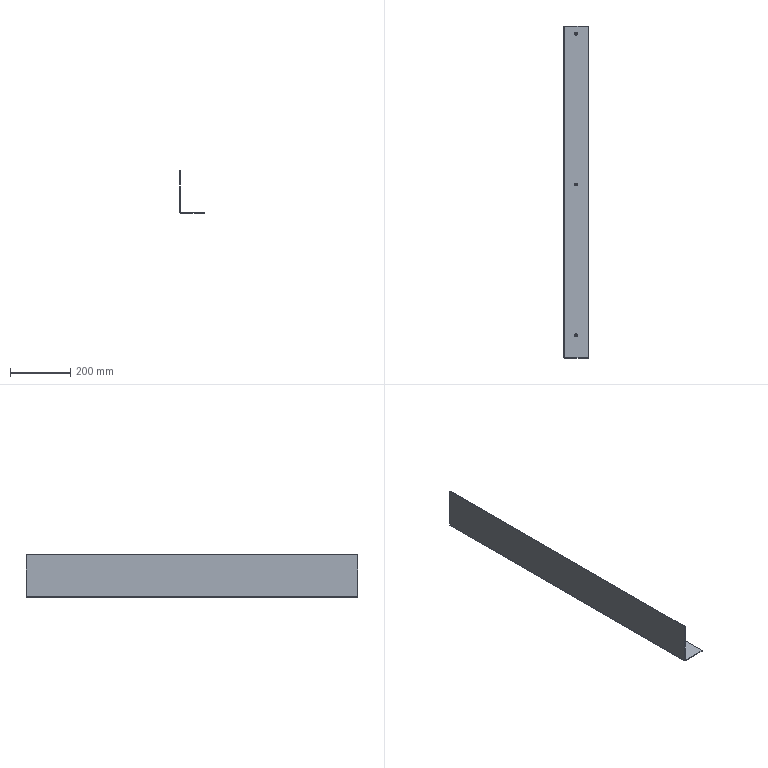Part | STEP file | PN_0006 Partition plate | 1 solid | 16 faces | box 82 x 1100 x 140 mm | volume 481847 mm3 | plane 8 | cone 6 | cylinder 2 | commonest cylinder face diameters 2 x1 6 x1
STEP:
#1=CARTESIAN_POINT('',(0.,0.,0.));
#2=DIRECTION('',(0.,0.,1.));
#3=DIRECTION('',(1.,0.,0.));
#4=AXIS2_PLACEMENT_3D('',#1,#2,#3);
#5=CARTESIAN_POINT('',(43.7,525.,0.));
#6=VERTEX_POINT('',#5);
#7=CARTESIAN_POINT('',(45.7,525.,2.));
#8=VERTEX_POINT('',#7);
#9=CARTESIAN_POINT('',(45.7,525.,2.));
#10=DIRECTION('',(0.7071,0.,0.7071));
#11=VECTOR('',#10,1.);
#12=LINE('',#9,#11);
#13=CARTESIAN_POINT('',(41.,525.,2.));
#14=DIRECTION('',(0.,0.,1.));
#15=DIRECTION('',(1.,0.,0.));
#16=AXIS2_PLACEMENT_3D('',#13,#14,#15);
#17=CONICAL_SURFACE('',#16,4.7,0.7854);
#18=CARTESIAN_POINT('',(6.283,0.));
#19=DIRECTION('',(0.,1.));
#20=VECTOR('',#19,1.);
#21=LINE('',#18,#20);
#22=(GEOMETRIC_REPRESENTATION_CONTEXT(2)PARAMETRIC_REPRESENTATION_CONTEXT()REPRESENTATION_CONTEXT('',''));
#23=DEFINITIONAL_REPRESENTATION('',(#21),#22);
#24=PCURVE('',#17,#23);
#25=CARTESIAN_POINT('',(41.,525.,2.));
#26=DIRECTION('',(0.,0.,1.));
#27=DIRECTION('',(1.,0.,0.));
#28=AXIS2_PLACEMENT_3D('',#25,#26,#27);
#29=CONICAL_SURFACE('',#28,4.7,0.7854);
#30=CARTESIAN_POINT('',(0.,0.));
#31=DIRECTION('',(0.,1.));
#32=VECTOR('',#31,1.);
#33=LINE('',#30,#32);
#34=(GEOMETRIC_REPRESENTATION_CONTEXT(2)PARAMETRIC_REPRESENTATION_CONTEXT()REPRESENTATION_CONTEXT('',''));
#35=DEFINITIONAL_REPRESENTATION('',(#33),#34);
#36=PCURVE('',#29,#35);
#37=SURFACE_CURVE('',#12,(#24,#36),.PCURVE_S1.);
#38=EDGE_CURVE('',#6,#8,#37,.T.);
#39=ORIENTED_EDGE('',*,*,#38,.T.);
#40=CARTESIAN_POINT('',(36.3,525.,2.));
#41=VERTEX_POINT('',#40);
#42=CARTESIAN_POINT('',(41.,525.,2.));
#43=DIRECTION('',(0.,0.,1.));
#44=DIRECTION('',(1.,0.,0.));
#45=AXIS2_PLACEMENT_3D('',#42,#43,#44);
#46=CIRCLE('',#45,4.7);
#47=CARTESIAN_POINT('',(0.,0.));
#48=DIRECTION('',(1.,0.));
#49=VECTOR('',#48,1.);
#50=LINE('',#47,#49);
#51=(GEOMETRIC_REPRESENTATION_CONTEXT(2)PARAMETRIC_REPRESENTATION_CONTEXT()REPRESENTATION_CONTEXT('',''));
#52=DEFINITIONAL_REPRESENTATION('',(#50),#51);
#53=PCURVE('',#17,#52);
#54=CARTESIAN_POINT('',(82.,550.,2.));
#55=DIRECTION('',(0.,0.,-1.));
#56=DIRECTION('',(-1.,0.,0.));
#57=AXIS2_PLACEMENT_3D('',#54,#55,#56);
#58=PLANE('',#57);
#59=CARTESIAN_POINT('',(36.3,-25.));
#60=CARTESIAN_POINT('',(36.3,-16.859));
#61=CARTESIAN_POINT('',(43.35,-20.93));
#62=CARTESIAN_POINT('',(50.4,-25.));
#63=CARTESIAN_POINT('',(43.35,-29.07));
#64=CARTESIAN_POINT('',(36.3,-33.141));
#65=CARTESIAN_POINT('',(36.3,-25.));
#66=(BOUNDED_CURVE()B_SPLINE_CURVE(2,(#59,#60,#61,#62,#63,#64,#65),.UNSPECIFIED.,.T.,.F.)B_SPLINE_CURVE_WITH_KNOTS((1,2,2,2,2,1),(-2.094,0.,2.094,4.189,6.283,8.378),.UNSPECIFIED.)CURVE()GEOMETRIC_REPRESENTATION_ITEM()RATIONAL_B_SPLINE_CURVE((1.,0.5,1.,0.5,1.,0.5,1.))REPRESENTATION_ITEM(''));
#67=(GEOMETRIC_REPRESENTATION_CONTEXT(2)PARAMETRIC_REPRESENTATION_CONTEXT()REPRESENTATION_CONTEXT('',''));
#68=DEFINITIONAL_REPRESENTATION('',(#66),#67);
#69=PCURVE('',#58,#68);
#70=SURFACE_CURVE('',#46,(#53,#69),.PCURVE_S1.);
#71=EDGE_CURVE('',#41,#8,#70,.T.);
#72=ORIENTED_EDGE('',*,*,#71,.F.);
#73=CARTESIAN_POINT('',(38.3,525.,0.));
#74=VERTEX_POINT('',#73);
#75=CARTESIAN_POINT('',(36.3,525.,2.));
#76=DIRECTION('',(-0.7071,0.,0.7071));
#77=VECTOR('',#76,1.);
#78=LINE('',#75,#77);
#79=CARTESIAN_POINT('',(3.142,0.));
#80=DIRECTION('',(0.,1.));
#81=VECTOR('',#80,1.);
#82=LINE('',#79,#81);
#83=(GEOMETRIC_REPRESENTATION_CONTEXT(2)PARAMETRIC_REPRESENTATION_CONTEXT()REPRESENTATION_CONTEXT('',''));
#84=DEFINITIONAL_REPRESENTATION('',(#82),#83);
#85=PCURVE('',#17,#84);
#86=CARTESIAN_POINT('',(3.142,0.));
#87=DIRECTION('',(0.,1.));
#88=VECTOR('',#87,1.);
#89=LINE('',#86,#88);
#90=(GEOMETRIC_REPRESENTATION_CONTEXT(2)PARAMETRIC_REPRESENTATION_CONTEXT()REPRESENTATION_CONTEXT('',''));
#91=DEFINITIONAL_REPRESENTATION('',(#89),#90);
#92=PCURVE('',#29,#91);
#93=SURFACE_CURVE('',#78,(#85,#92),.PCURVE_S1.);
#94=EDGE_CURVE('',#74,#41,#93,.T.);
#95=ORIENTED_EDGE('',*,*,#94,.F.);
#96=CARTESIAN_POINT('',(41.,525.,0.));
#97=DIRECTION('',(0.,0.,1.));
#98=DIRECTION('',(1.,0.,0.));
#99=AXIS2_PLACEMENT_3D('',#96,#97,#98);
#100=CIRCLE('',#99,2.7);
#101=CARTESIAN_POINT('',(0.,-2.));
#102=DIRECTION('',(1.,0.));
#103=VECTOR('',#102,1.);
#104=LINE('',#101,#103);
#105=(GEOMETRIC_REPRESENTATION_CONTEXT(2)PARAMETRIC_REPRESENTATION_CONTEXT()REPRESENTATION_CONTEXT('',''));
#106=DEFINITIONAL_REPRESENTATION('',(#104),#105);
#107=PCURVE('',#17,#106);
#108=CARTESIAN_POINT('',(3.,550.,0.));
#109=DIRECTION('',(0.,0.,1.));
#110=DIRECTION('',(1.,0.,0.));
#111=AXIS2_PLACEMENT_3D('',#108,#109,#110);
#112=PLANE('',#111);
#113=CARTESIAN_POINT('',(38.,-25.));
#114=DIRECTION('',(1.,0.));
#115=AXIS2_PLACEMENT_2D('',#113,#114);
#116=CIRCLE('',#115,2.7);
#117=(GEOMETRIC_REPRESENTATION_CONTEXT(2)PARAMETRIC_REPRESENTATION_CONTEXT()REPRESENTATION_CONTEXT('',''));
#118=DEFINITIONAL_REPRESENTATION('',(#116),#117);
#119=PCURVE('',#112,#118);
#120=SURFACE_CURVE('',#100,(#107,#119),.PCURVE_S1.);
#121=EDGE_CURVE('',#74,#6,#120,.T.);
#122=ORIENTED_EDGE('',*,*,#121,.T.);
#123=EDGE_LOOP('',(#39,#72,#95,#122));
#124=FACE_BOUND('',#123,.F.);
#125=ADVANCED_FACE('',(#124),#17,.F.);
#126=CARTESIAN_POINT('',(43.7,25.,0.));
#127=VERTEX_POINT('',#126);
#128=CARTESIAN_POINT('',(45.7,25.,2.));
#129=VERTEX_POINT('',#128);
#130=CARTESIAN_POINT('',(45.7,25.,2.));
#131=DIRECTION('',(0.7071,0.,0.7071));
#132=VECTOR('',#131,1.);
#133=LINE('',#130,#132);
#134=CARTESIAN_POINT('',(41.,25.,2.));
#135=DIRECTION('',(0.,0.,1.));
#136=DIRECTION('',(1.,0.,0.));
#137=AXIS2_PLACEMENT_3D('',#134,#135,#136);
#138=CONICAL_SURFACE('',#137,4.7,0.7854);
#139=CARTESIAN_POINT('',(6.283,0.));
#140=DIRECTION('',(0.,1.));
#141=VECTOR('',#140,1.);
#142=LINE('',#139,#141);
#143=(GEOMETRIC_REPRESENTATION_CONTEXT(2)PARAMETRIC_REPRESENTATION_CONTEXT()REPRESENTATION_CONTEXT('',''));
#144=DEFINITIONAL_REPRESENTATION('',(#142),#143);
#145=PCURVE('',#138,#144);
#146=CARTESIAN_POINT('',(41.,25.,2.));
#147=DIRECTION('',(0.,0.,1.));
#148=DIRECTION('',(1.,0.,0.));
#149=AXIS2_PLACEMENT_3D('',#146,#147,#148);
#150=CONICAL_SURFACE('',#149,4.7,0.7854);
#151=CARTESIAN_POINT('',(0.,0.));
#152=DIRECTION('',(0.,1.));
#153=VECTOR('',#152,1.);
#154=LINE('',#151,#153);
#155=(GEOMETRIC_REPRESENTATION_CONTEXT(2)PARAMETRIC_REPRESENTATION_CONTEXT()REPRESENTATION_CONTEXT('',''));
#156=DEFINITIONAL_REPRESENTATION('',(#154),#155);
#157=PCURVE('',#150,#156);
#158=SURFACE_CURVE('',#133,(#145,#157),.PCURVE_S1.);
#159=EDGE_CURVE('',#127,#129,#158,.T.);
#160=ORIENTED_EDGE('',*,*,#159,.T.);
#161=CARTESIAN_POINT('',(36.3,25.,2.));
#162=VERTEX_POINT('',#161);
#163=CARTESIAN_POINT('',(41.,25.,2.));
#164=DIRECTION('',(0.,0.,1.));
#165=DIRECTION('',(1.,0.,0.));
#166=AXIS2_PLACEMENT_3D('',#163,#164,#165);
#167=CIRCLE('',#166,4.7);
#168=CARTESIAN_POINT('',(0.,0.));
#169=DIRECTION('',(1.,0.));
#170=VECTOR('',#169,1.);
#171=LINE('',#168,#170);
#172=(GEOMETRIC_REPRESENTATION_CONTEXT(2)PARAMETRIC_REPRESENTATION_CONTEXT()REPRESENTATION_CONTEXT('',''));
#173=DEFINITIONAL_REPRESENTATION('',(#171),#172);
#174=PCURVE('',#138,#173);
#175=CARTESIAN_POINT('',(36.3,-525.));
#176=CARTESIAN_POINT('',(36.3,-516.859));
#177=CARTESIAN_POINT('',(43.35,-520.93));
#178=CARTESIAN_POINT('',(50.4,-525.));
#179=CARTESIAN_POINT('',(43.35,-529.07));
#180=CARTESIAN_POINT('',(36.3,-533.141));
#181=CARTESIAN_POINT('',(36.3,-525.));
#182=(BOUNDED_CURVE()B_SPLINE_CURVE(2,(#175,#176,#177,#178,#179,#180,#181),.UNSPECIFIED.,.T.,.F.)B_SPLINE_CURVE_WITH_KNOTS((1,2,2,2,2,1),(-2.094,0.,2.094,4.189,6.283,8.378),.UNSPECIFIED.)CURVE()GEOMETRIC_REPRESENTATION_ITEM()RATIONAL_B_SPLINE_CURVE((1.,0.5,1.,0.5,1.,0.5,1.))REPRESENTATION_ITEM(''));
#183=(GEOMETRIC_REPRESENTATION_CONTEXT(2)PARAMETRIC_REPRESENTATION_CONTEXT()REPRESENTATION_CONTEXT('',''));
#184=DEFINITIONAL_REPRESENTATION('',(#182),#183);
#185=PCURVE('',#58,#184);
#186=SURFACE_CURVE('',#167,(#174,#185),.PCURVE_S1.);
#187=EDGE_CURVE('',#162,#129,#186,.T.);
#188=ORIENTED_EDGE('',*,*,#187,.F.);
#189=CARTESIAN_POINT('',(38.3,25.,0.));
#190=VERTEX_POINT('',#189);
#191=CARTESIAN_POINT('',(36.3,25.,2.));
#192=DIRECTION('',(-0.7071,0.,0.7071));
#193=VECTOR('',#192,1.);
#194=LINE('',#191,#193);
#195=CARTESIAN_POINT('',(3.142,0.));
#196=DIRECTION('',(0.,1.));
#197=VECTOR('',#196,1.);
#198=LINE('',#195,#197);
#199=(GEOMETRIC_REPRESENTATION_CONTEXT(2)PARAMETRIC_REPRESENTATION_CONTEXT()REPRESENTATION_CONTEXT('',''));
#200=DEFINITIONAL_REPRESENTATION('',(#198),#199);
#201=PCURVE('',#138,#200);
#202=CARTESIAN_POINT('',(3.142,0.));
#203=DIRECTION('',(0.,1.));
#204=VECTOR('',#203,1.);
#205=LINE('',#202,#204);
#206=(GEOMETRIC_REPRESENTATION_CONTEXT(2)PARAMETRIC_REPRESENTATION_CONTEXT()REPRESENTATION_CONTEXT('',''));
#207=DEFINITIONAL_REPRESENTATION('',(#205),#206);
#208=PCURVE('',#150,#207);
#209=SURFACE_CURVE('',#194,(#201,#208),.PCURVE_S1.);
#210=EDGE_CURVE('',#190,#162,#209,.T.);
#211=ORIENTED_EDGE('',*,*,#210,.F.);
#212=CARTESIAN_POINT('',(41.,25.,0.));
#213=DIRECTION('',(0.,0.,1.));
#214=DIRECTION('',(1.,0.,0.));
#215=AXIS2_PLACEMENT_3D('',#212,#213,#214);
#216=CIRCLE('',#215,2.7);
#217=CARTESIAN_POINT('',(0.,-2.));
#218=DIRECTION('',(1.,0.));
#219=VECTOR('',#218,1.);
#220=LINE('',#217,#219);
#221=(GEOMETRIC_REPRESENTATION_CONTEXT(2)PARAMETRIC_REPRESENTATION_CONTEXT()REPRESENTATION_CONTEXT('',''));
#222=DEFINITIONAL_REPRESENTATION('',(#220),#221);
#223=PCURVE('',#138,#222);
#224=CARTESIAN_POINT('',(38.,-525.));
#225=DIRECTION('',(1.,0.));
#226=AXIS2_PLACEMENT_2D('',#224,#225);
#227=CIRCLE('',#226,2.7);
#228=(GEOMETRIC_REPRESENTATION_CONTEXT(2)PARAMETRIC_REPRESENTATION_CONTEXT()REPRESENTATION_CONTEXT('',''));
#229=DEFINITIONAL_REPRESENTATION('',(#227),#228);
#230=PCURVE('',#112,#229);
#231=SURFACE_CURVE('',#216,(#223,#230),.PCURVE_S1.);
#232=EDGE_CURVE('',#190,#127,#231,.T.);
#233=ORIENTED_EDGE('',*,*,#232,.T.);
#234=EDGE_LOOP('',(#160,#188,#211,#233));
#235=FACE_BOUND('',#234,.F.);
#236=ADVANCED_FACE('',(#235),#138,.F.);
#237=CARTESIAN_POINT('',(43.7,-475.,0.));
#238=VERTEX_POINT('',#237);
#239=CARTESIAN_POINT('',(45.7,-475.,2.));
#240=VERTEX_POINT('',#239);
#241=CARTESIAN_POINT('',(45.7,-475.,2.));
#242=DIRECTION('',(0.7071,0.,0.7071));
#243=VECTOR('',#242,1.);
#244=LINE('',#241,#243);
#245=CARTESIAN_POINT('',(41.,-475.,2.));
#246=DIRECTION('',(0.,0.,1.));
#247=DIRECTION('',(1.,0.,0.));
#248=AXIS2_PLACEMENT_3D('',#245,#246,#247);
#249=CONICAL_SURFACE('',#248,4.7,0.7854);
#250=CARTESIAN_POINT('',(6.283,0.));
#251=DIRECTION('',(0.,1.));
#252=VECTOR('',#251,1.);
#253=LINE('',#250,#252);
#254=(GEOMETRIC_REPRESENTATION_CONTEXT(2)PARAMETRIC_REPRESENTATION_CONTEXT()REPRESENTATION_CONTEXT('',''));
#255=DEFINITIONAL_REPRESENTATION('',(#253),#254);
#256=PCURVE('',#249,#255);
#257=CARTESIAN_POINT('',(41.,-475.,2.));
#258=DIRECTION('',(0.,0.,1.));
#259=DIRECTION('',(1.,0.,0.));
#260=AXIS2_PLACEMENT_3D('',#257,#258,#259);
#261=CONICAL_SURFACE('',#260,4.7,0.7854);
#262=CARTESIAN_POINT('',(0.,0.));
#263=DIRECTION('',(0.,1.));
#264=VECTOR('',#263,1.);
#265=LINE('',#262,#264);
#266=(GEOMETRIC_REPRESENTATION_CONTEXT(2)PARAMETRIC_REPRESENTATION_CONTEXT()REPRESENTATION_CONTEXT('',''));
#267=DEFINITIONAL_REPRESENTATION('',(#265),#266);
#268=PCURVE('',#261,#267);
#269=SURFACE_CURVE('',#244,(#256,#268),.PCURVE_S1.);
#270=EDGE_CURVE('',#238,#240,#269,.T.);
#271=ORIENTED_EDGE('',*,*,#270,.T.);
#272=CARTESIAN_POINT('',(36.3,-475.,2.));
#273=VERTEX_POINT('',#272);
#274=CARTESIAN_POINT('',(41.,-475.,2.));
#275=DIRECTION('',(0.,0.,1.));
#276=DIRECTION('',(1.,0.,0.));
#277=AXIS2_PLACEMENT_3D('',#274,#275,#276);
#278=CIRCLE('',#277,4.7);
#279=CARTESIAN_POINT('',(0.,0.));
#280=DIRECTION('',(1.,0.));
#281=VECTOR('',#280,1.);
#282=LINE('',#279,#281);
#283=(GEOMETRIC_REPRESENTATION_CONTEXT(2)PARAMETRIC_REPRESENTATION_CONTEXT()REPRESENTATION_CONTEXT('',''));
#284=DEFINITIONAL_REPRESENTATION('',(#282),#283);
#285=PCURVE('',#249,#284);
#286=CARTESIAN_POINT('',(36.3,-1025.));
#287=CARTESIAN_POINT('',(36.3,-1016.859));
#288=CARTESIAN_POINT('',(43.35,-1020.93));
#289=CARTESIAN_POINT('',(50.4,-1025.));
#290=CARTESIAN_POINT('',(43.35,-1029.07));
#291=CARTESIAN_POINT('',(36.3,-1033.141));
#292=CARTESIAN_POINT('',(36.3,-1025.));
#293=(BOUNDED_CURVE()B_SPLINE_CURVE(2,(#286,#287,#288,#289,#290,#291,#292),.UNSPECIFIED.,.T.,.F.)B_SPLINE_CURVE_WITH_KNOTS((1,2,2,2,2,1),(-2.094,0.,2.094,4.189,6.283,8.378),.UNSPECIFIED.)CURVE()GEOMETRIC_REPRESENTATION_ITEM()RATIONAL_B_SPLINE_CURVE((1.,0.5,1.,0.5,1.,0.5,1.))REPRESENTATION_ITEM(''));
#294=(GEOMETRIC_REPRESENTATION_CONTEXT(2)PARAMETRIC_REPRESENTATION_CONTEXT()REPRESENTATION_CONTEXT('',''));
#295=DEFINITIONAL_REPRESENTATION('',(#293),#294);
#296=PCURVE('',#58,#295);
#297=SURFACE_CURVE('',#278,(#285,#296),.PCURVE_S1.);
#298=EDGE_CURVE('',#273,#240,#297,.T.);
#299=ORIENTED_EDGE('',*,*,#298,.F.);
#300=CARTESIAN_POINT('',(38.3,-475.,0.));
#301=VERTEX_POINT('',#300);
#302=CARTESIAN_POINT('',(36.3,-475.,2.));
#303=DIRECTION('',(-0.7071,0.,0.7071));
#304=VECTOR('',#303,1.);
#305=LINE('',#302,#304);
#306=CARTESIAN_POINT('',(3.142,0.));
#307=DIRECTION('',(0.,1.));
#308=VECTOR('',#307,1.);
#309=LINE('',#306,#308);
#310=(GEOMETRIC_REPRESENTATION_CONTEXT(2)PARAMETRIC_REPRESENTATION_CONTEXT()REPRESENTATION_CONTEXT('',''));
#311=DEFINITIONAL_REPRESENTATION('',(#309),#310);
#312=PCURVE('',#249,#311);
#313=CARTESIAN_POINT('',(3.142,0.));
#314=DIRECTION('',(0.,1.));
#315=VECTOR('',#314,1.);
#316=LINE('',#313,#315);
#317=(GEOMETRIC_REPRESENTATION_CONTEXT(2)PARAMETRIC_REPRESENTATION_CONTEXT()REPRESENTATION_CONTEXT('',''));
#318=DEFINITIONAL_REPRESENTATION('',(#316),#317);
#319=PCURVE('',#261,#318);
#320=SURFACE_CURVE('',#305,(#312,#319),.PCURVE_S1.);
#321=EDGE_CURVE('',#301,#273,#320,.T.);
#322=ORIENTED_EDGE('',*,*,#321,.F.);
#323=CARTESIAN_POINT('',(41.,-475.,0.));
#324=DIRECTION('',(0.,0.,1.));
#325=DIRECTION('',(1.,0.,0.));
#326=AXIS2_PLACEMENT_3D('',#323,#324,#325);
#327=CIRCLE('',#326,2.7);
#328=CARTESIAN_POINT('',(0.,-2.));
#329=DIRECTION('',(1.,0.));
#330=VECTOR('',#329,1.);
#331=LINE('',#328,#330);
#332=(GEOMETRIC_REPRESENTATION_CONTEXT(2)PARAMETRIC_REPRESENTATION_CONTEXT()REPRESENTATION_CONTEXT('',''));
#333=DEFINITIONAL_REPRESENTATION('',(#331),#332);
#334=PCURVE('',#249,#333);
#335=CARTESIAN_POINT('',(38.,-1025.));
#336=DIRECTION('',(1.,0.));
#337=AXIS2_PLACEMENT_2D('',#335,#336);
#338=CIRCLE('',#337,2.7);
#339=(GEOMETRIC_REPRESENTATION_CONTEXT(2)PARAMETRIC_REPRESENTATION_CONTEXT()REPRESENTATION_CONTEXT('',''));
#340=DEFINITIONAL_REPRESENTATION('',(#338),#339);
#341=PCURVE('',#112,#340);
#342=SURFACE_CURVE('',#327,(#334,#341),.PCURVE_S1.);
#343=EDGE_CURVE('',#301,#238,#342,.T.);
#344=ORIENTED_EDGE('',*,*,#343,.T.);
#345=EDGE_LOOP('',(#271,#299,#322,#344));
#346=FACE_BOUND('',#345,.F.);
#347=ADVANCED_FACE('',(#346),#249,.F.);
#348=CARTESIAN_POINT('',(41.,525.,0.));
#349=DIRECTION('',(0.,0.,1.));
#350=DIRECTION('',(1.,0.,0.));
#351=AXIS2_PLACEMENT_3D('',#348,#349,#350);
#352=CIRCLE('',#351,2.7);
#353=CARTESIAN_POINT('',(38.,-25.));
#354=DIRECTION('',(1.,0.));
#355=AXIS2_PLACEMENT_2D('',#353,#354);
#356=CIRCLE('',#355,2.7);
#357=(GEOMETRIC_REPRESENTATION_CONTEXT(2)PARAMETRIC_REPRESENTATION_CONTEXT()REPRESENTATION_CONTEXT('',''));
#358=DEFINITIONAL_REPRESENTATION('',(#356),#357);
#359=PCURVE('',#112,#358);
#360=CARTESIAN_POINT('',(0.,-2.));
#361=DIRECTION('',(1.,0.));
#362=VECTOR('',#361,1.);
#363=LINE('',#360,#362);
#364=(GEOMETRIC_REPRESENTATION_CONTEXT(2)PARAMETRIC_REPRESENTATION_CONTEXT()REPRESENTATION_CONTEXT('',''));
#365=DEFINITIONAL_REPRESENTATION('',(#363),#364);
#366=PCURVE('',#29,#365);
#367=SURFACE_CURVE('',#352,(#359,#366),.PCURVE_S1.);
#368=EDGE_CURVE('',#6,#74,#367,.T.);
#369=ORIENTED_EDGE('',*,*,#368,.T.);
#370=ORIENTED_EDGE('',*,*,#121,.T.);
#371=EDGE_LOOP('',(#369,#370));
#372=FACE_BOUND('',#371,.T.);
#373=CARTESIAN_POINT('',(41.,25.,0.));
#374=DIRECTION('',(0.,0.,1.));
#375=DIRECTION('',(1.,0.,0.));
#376=AXIS2_PLACEMENT_3D('',#373,#374,#375);
#377=CIRCLE('',#376,2.7);
#378=CARTESIAN_POINT('',(38.,-525.));
#379=DIRECTION('',(1.,0.));
#380=AXIS2_PLACEMENT_2D('',#378,#379);
#381=CIRCLE('',#380,2.7);
#382=(GEOMETRIC_REPRESENTATION_CONTEXT(2)PARAMETRIC_REPRESENTATION_CONTEXT()REPRESENTATION_CONTEXT('',''));
#383=DEFINITIONAL_REPRESENTATION('',(#381),#382);
#384=PCURVE('',#112,#383);
#385=CARTESIAN_POINT('',(0.,-2.));
#386=DIRECTION('',(1.,0.));
#387=VECTOR('',#386,1.);
#388=LINE('',#385,#387);
#389=(GEOMETRIC_REPRESENTATION_CONTEXT(2)PARAMETRIC_REPRESENTATION_CONTEXT()REPRESENTATION_CONTEXT('',''));
#390=DEFINITIONAL_REPRESENTATION('',(#388),#389);
#391=PCURVE('',#150,#390);
#392=SURFACE_CURVE('',#377,(#384,#391),.PCURVE_S1.);
#393=EDGE_CURVE('',#127,#190,#392,.T.);
#394=ORIENTED_EDGE('',*,*,#393,.T.);
#395=ORIENTED_EDGE('',*,*,#232,.T.);
#396=EDGE_LOOP('',(#394,#395));
#397=FACE_BOUND('',#396,.T.);
#398=CARTESIAN_POINT('',(41.,-475.,0.));
#399=DIRECTION('',(0.,0.,1.));
#400=DIRECTION('',(1.,0.,0.));
#401=AXIS2_PLACEMENT_3D('',#398,#399,#400);
#402=CIRCLE('',#401,2.7);
#403=CARTESIAN_POINT('',(38.,-1025.));
#404=DIRECTION('',(1.,0.));
#405=AXIS2_PLACEMENT_2D('',#403,#404);
#406=CIRCLE('',#405,2.7);
#407=(GEOMETRIC_REPRESENTATION_CONTEXT(2)PARAMETRIC_REPRESENTATION_CONTEXT()REPRESENTATION_CONTEXT('',''));
#408=DEFINITIONAL_REPRESENTATION('',(#406),#407);
#409=PCURVE('',#112,#408);
#410=CARTESIAN_POINT('',(0.,-2.));
#411=DIRECTION('',(1.,0.));
#412=VECTOR('',#411,1.);
#413=LINE('',#410,#412);
#414=(GEOMETRIC_REPRESENTATION_CONTEXT(2)PARAMETRIC_REPRESENTATION_CONTEXT()REPRESENTATION_CONTEXT('',''));
#415=DEFINITIONAL_REPRESENTATION('',(#413),#414);
#416=PCURVE('',#261,#415);
#417=SURFACE_CURVE('',#402,(#409,#416),.PCURVE_S1.);
#418=EDGE_CURVE('',#238,#301,#417,.T.);
#419=ORIENTED_EDGE('',*,*,#418,.T.);
#420=ORIENTED_EDGE('',*,*,#343,.T.);
#421=EDGE_LOOP('',(#419,#420));
#422=FACE_BOUND('',#421,.T.);
#423=CARTESIAN_POINT('',(82.,-550.,0.));
#424=VERTEX_POINT('',#423);
#425=CARTESIAN_POINT('',(3.,-550.,0.));
#426=VERTEX_POINT('',#425);
#427=CARTESIAN_POINT('',(3.,-550.,0.));
#428=DIRECTION('',(-1.,0.,0.));
#429=VECTOR('',#428,1.);
#430=LINE('',#427,#429);
#431=CARTESIAN_POINT('',(0.,-1100.));
#432=DIRECTION('',(-1.,0.));
#433=VECTOR('',#432,1.);
#434=LINE('',#431,#433);
#435=(GEOMETRIC_REPRESENTATION_CONTEXT(2)PARAMETRIC_REPRESENTATION_CONTEXT()REPRESENTATION_CONTEXT('',''));
#436=DEFINITIONAL_REPRESENTATION('',(#434),#435);
#437=PCURVE('',#112,#436);
#438=CARTESIAN_POINT('',(3.,-550.,3.));
#439=DIRECTION('',(0.,-1.,0.));
#440=DIRECTION('',(0.,0.,-1.));
#441=AXIS2_PLACEMENT_3D('',#438,#439,#440);
#442=PLANE('',#441);
#443=CARTESIAN_POINT('',(3.,0.));
#444=DIRECTION('',(0.,-1.));
#445=VECTOR('',#444,1.);
#446=LINE('',#443,#445);
#447=(GEOMETRIC_REPRESENTATION_CONTEXT(2)PARAMETRIC_REPRESENTATION_CONTEXT()REPRESENTATION_CONTEXT('',''));
#448=DEFINITIONAL_REPRESENTATION('',(#446),#447);
#449=PCURVE('',#442,#448);
#450=SURFACE_CURVE('',#430,(#437,#449),.PCURVE_S1.);
#451=EDGE_CURVE('',#424,#426,#450,.T.);
#452=ORIENTED_EDGE('',*,*,#451,.T.);
#453=CARTESIAN_POINT('',(3.,550.,0.));
#454=VERTEX_POINT('',#453);
#455=CARTESIAN_POINT('',(3.,550.,0.));
#456=DIRECTION('',(0.,-1.,0.));
#457=VECTOR('',#456,1.);
#458=LINE('',#455,#457);
#459=CARTESIAN_POINT('',(0.,0.));
#460=DIRECTION('',(0.,-1.));
#461=VECTOR('',#460,1.);
#462=LINE('',#459,#461);
#463=(GEOMETRIC_REPRESENTATION_CONTEXT(2)PARAMETRIC_REPRESENTATION_CONTEXT()REPRESENTATION_CONTEXT('',''));
#464=DEFINITIONAL_REPRESENTATION('',(#462),#463);
#465=PCURVE('',#112,#464);
#466=CARTESIAN_POINT('',(3.,550.,3.));
#467=DIRECTION('',(0.,-1.,0.));
#468=DIRECTION('',(0.,0.,-1.));
#469=AXIS2_PLACEMENT_3D('',#466,#467,#468);
#470=CYLINDRICAL_SURFACE('',#469,3.);
#471=CARTESIAN_POINT('',(6.283,0.));
#472=DIRECTION('',(0.,1.));
#473=VECTOR('',#472,1.);
#474=LINE('',#471,#473);
#475=(GEOMETRIC_REPRESENTATION_CONTEXT(2)PARAMETRIC_REPRESENTATION_CONTEXT()REPRESENTATION_CONTEXT('',''));
#476=DEFINITIONAL_REPRESENTATION('',(#474),#475);
#477=PCURVE('',#470,#476);
#478=SURFACE_CURVE('',#458,(#465,#477),.PCURVE_S1.);
#479=EDGE_CURVE('',#454,#426,#478,.T.);
#480=ORIENTED_EDGE('',*,*,#479,.F.);
#481=CARTESIAN_POINT('',(82.,550.,0.));
#482=VERTEX_POINT('',#481);
#483=CARTESIAN_POINT('',(3.,550.,0.));
#484=DIRECTION('',(-1.,0.,0.));
#485=VECTOR('',#484,1.);
#486=LINE('',#483,#485);
#487=CARTESIAN_POINT('',(0.,0.));
#488=DIRECTION('',(-1.,0.));
#489=VECTOR('',#488,1.);
#490=LINE('',#487,#489);
#491=(GEOMETRIC_REPRESENTATION_CONTEXT(2)PARAMETRIC_REPRESENTATION_CONTEXT()REPRESENTATION_CONTEXT('',''));
#492=DEFINITIONAL_REPRESENTATION('',(#490),#491);
#493=PCURVE('',#112,#492);
#494=CARTESIAN_POINT('',(3.,550.,3.));
#495=DIRECTION('',(0.,-1.,0.));
#496=DIRECTION('',(0.,0.,-1.));
#497=AXIS2_PLACEMENT_3D('',#494,#495,#496);
#498=PLANE('',#497);
#499=CARTESIAN_POINT('',(3.,0.));
#500=DIRECTION('',(0.,-1.));
#501=VECTOR('',#500,1.);
#502=LINE('',#499,#501);
#503=(GEOMETRIC_REPRESENTATION_CONTEXT(2)PARAMETRIC_REPRESENTATION_CONTEXT()REPRESENTATION_CONTEXT('',''));
#504=DEFINITIONAL_REPRESENTATION('',(#502),#503);
#505=PCURVE('',#498,#504);
#506=SURFACE_CURVE('',#486,(#493,#505),.PCURVE_S1.);
#507=EDGE_CURVE('',#482,#454,#506,.T.);
#508=ORIENTED_EDGE('',*,*,#507,.F.);
#509=CARTESIAN_POINT('',(82.,550.,0.));
#510=DIRECTION('',(0.,-1.,0.));
#511=VECTOR('',#510,1.);
#512=LINE('',#509,#511);
#513=CARTESIAN_POINT('',(79.,0.));
#514=DIRECTION('',(0.,-1.));
#515=VECTOR('',#514,1.);
#516=LINE('',#513,#515);
#517=(GEOMETRIC_REPRESENTATION_CONTEXT(2)PARAMETRIC_REPRESENTATION_CONTEXT()REPRESENTATION_CONTEXT('',''));
#518=DEFINITIONAL_REPRESENTATION('',(#516),#517);
#519=PCURVE('',#112,#518);
#520=CARTESIAN_POINT('',(82.,550.,0.));
#521=DIRECTION('',(-1.,0.,0.));
#522=DIRECTION('',(0.,0.,1.));
#523=AXIS2_PLACEMENT_3D('',#520,#521,#522);
#524=PLANE('',#523);
#525=CARTESIAN_POINT('',(0.,0.));
#526=DIRECTION('',(0.,-1.));
#527=VECTOR('',#526,1.);
#528=LINE('',#525,#527);
#529=(GEOMETRIC_REPRESENTATION_CONTEXT(2)PARAMETRIC_REPRESENTATION_CONTEXT()REPRESENTATION_CONTEXT('',''));
#530=DEFINITIONAL_REPRESENTATION('',(#528),#529);
#531=PCURVE('',#524,#530);
#532=SURFACE_CURVE('',#512,(#519,#531),.PCURVE_S1.);
#533=EDGE_CURVE('',#482,#424,#532,.T.);
#534=ORIENTED_EDGE('',*,*,#533,.T.);
#535=EDGE_LOOP('',(#452,#480,#508,#534));
#536=FACE_BOUND('',#535,.T.);
#537=ADVANCED_FACE('',(#372,#397,#422,#536),#112,.F.);
#538=CARTESIAN_POINT('',(0.,-550.,140.));
#539=VERTEX_POINT('',#538);
#540=CARTESIAN_POINT('',(2.,-550.,140.));
#541=VERTEX_POINT('',#540);
#542=CARTESIAN_POINT('',(2.,-550.,140.));
#543=DIRECTION('',(1.,0.,0.));
#544=VECTOR('',#543,1.);
#545=LINE('',#542,#544);
#546=CARTESIAN_POINT('',(2.,550.,140.));
#547=DIRECTION('',(0.,0.,-1.));
#548=DIRECTION('',(-1.,0.,0.));
#549=AXIS2_PLACEMENT_3D('',#546,#547,#548);
#550=PLANE('',#549);
#551=CARTESIAN_POINT('',(0.,-1100.));
#552=DIRECTION('',(-1.,0.));
#553=VECTOR('',#552,1.);
#554=LINE('',#551,#553);
#555=(GEOMETRIC_REPRESENTATION_CONTEXT(2)PARAMETRIC_REPRESENTATION_CONTEXT()REPRESENTATION_CONTEXT('',''));
#556=DEFINITIONAL_REPRESENTATION('',(#554),#555);
#557=PCURVE('',#550,#556);
#558=CARTESIAN_POINT('',(-137.,-1.));
#559=DIRECTION('',(0.,1.));
#560=VECTOR('',#559,1.);
#561=LINE('',#558,#560);
#562=(GEOMETRIC_REPRESENTATION_CONTEXT(2)PARAMETRIC_REPRESENTATION_CONTEXT()REPRESENTATION_CONTEXT('',''));
#563=DEFINITIONAL_REPRESENTATION('',(#561),#562);
#564=PCURVE('',#442,#563);
#565=SURFACE_CURVE('',#545,(#557,#564),.PCURVE_S1.);
#566=EDGE_CURVE('',#539,#541,#565,.T.);
#567=ORIENTED_EDGE('',*,*,#566,.T.);
#568=CARTESIAN_POINT('',(2.,550.,140.));
#569=VERTEX_POINT('',#568);
#570=CARTESIAN_POINT('',(2.,550.,140.));
#571=DIRECTION('',(0.,-1.,0.));
#572=VECTOR('',#571,1.);
#573=LINE('',#570,#572);
#574=CARTESIAN_POINT('',(0.,0.));
#575=DIRECTION('',(0.,-1.));
#576=VECTOR('',#575,1.);
#577=LINE('',#574,#576);
#578=(GEOMETRIC_REPRESENTATION_CONTEXT(2)PARAMETRIC_REPRESENTATION_CONTEXT()REPRESENTATION_CONTEXT('',''));
#579=DEFINITIONAL_REPRESENTATION('',(#577),#578);
#580=PCURVE('',#550,#579);
#581=CARTESIAN_POINT('',(2.,550.,3.));
#582=DIRECTION('',(-1.,0.,0.));
#583=DIRECTION('',(0.,0.,1.));
#584=AXIS2_PLACEMENT_3D('',#581,#582,#583);
#585=PLANE('',#584);
#586=CARTESIAN_POINT('',(137.,0.));
#587=DIRECTION('',(0.,-1.));
#588=VECTOR('',#587,1.);
#589=LINE('',#586,#588);
#590=(GEOMETRIC_REPRESENTATION_CONTEXT(2)PARAMETRIC_REPRESENTATION_CONTEXT()REPRESENTATION_CONTEXT('',''));
#591=DEFINITIONAL_REPRESENTATION('',(#589),#590);
#592=PCURVE('',#585,#591);
#593=SURFACE_CURVE('',#573,(#580,#592),.PCURVE_S1.);
#594=EDGE_CURVE('',#569,#541,#593,.T.);
#595=ORIENTED_EDGE('',*,*,#594,.F.);
#596=CARTESIAN_POINT('',(0.,550.,140.));
#597=VERTEX_POINT('',#596);
#598=CARTESIAN_POINT('',(2.,550.,140.));
#599=DIRECTION('',(1.,0.,0.));
#600=VECTOR('',#599,1.);
#601=LINE('',#598,#600);
#602=CARTESIAN_POINT('',(0.,0.));
#603=DIRECTION('',(-1.,0.));
#604=VECTOR('',#603,1.);
#605=LINE('',#602,#604);
#606=(GEOMETRIC_REPRESENTATION_CONTEXT(2)PARAMETRIC_REPRESENTATION_CONTEXT()REPRESENTATION_CONTEXT('',''));
#607=DEFINITIONAL_REPRESENTATION('',(#605),#606);
#608=PCURVE('',#550,#607);
#609=CARTESIAN_POINT('',(-137.,-1.));
#610=DIRECTION('',(0.,1.));
#611=VECTOR('',#610,1.);
#612=LINE('',#609,#611);
#613=(GEOMETRIC_REPRESENTATION_CONTEXT(2)PARAMETRIC_REPRESENTATION_CONTEXT()REPRESENTATION_CONTEXT('',''));
#614=DEFINITIONAL_REPRESENTATION('',(#612),#613);
#615=PCURVE('',#498,#614);
#616=SURFACE_CURVE('',#601,(#608,#615),.PCURVE_S1.);
#617=EDGE_CURVE('',#597,#569,#616,.T.);
#618=ORIENTED_EDGE('',*,*,#617,.F.);
#619=CARTESIAN_POINT('',(0.,550.,140.));
#620=DIRECTION('',(0.,-1.,0.));
#621=VECTOR('',#620,1.);
#622=LINE('',#619,#621);
#623=CARTESIAN_POINT('',(2.,0.));
#624=DIRECTION('',(0.,-1.));
#625=VECTOR('',#624,1.);
#626=LINE('',#623,#625);
#627=(GEOMETRIC_REPRESENTATION_CONTEXT(2)PARAMETRIC_REPRESENTATION_CONTEXT()REPRESENTATION_CONTEXT('',''));
#628=DEFINITIONAL_REPRESENTATION('',(#626),#627);
#629=PCURVE('',#550,#628);
#630=CARTESIAN_POINT('',(0.,550.,140.));
#631=DIRECTION('',(1.,0.,0.));
#632=DIRECTION('',(0.,0.,-1.));
#633=AXIS2_PLACEMENT_3D('',#630,#631,#632);
#634=PLANE('',#633);
#635=CARTESIAN_POINT('',(0.,0.));
#636=DIRECTION('',(0.,-1.));
#637=VECTOR('',#636,1.);
#638=LINE('',#635,#637);
#639=(GEOMETRIC_REPRESENTATION_CONTEXT(2)PARAMETRIC_REPRESENTATION_CONTEXT()REPRESENTATION_CONTEXT('',''));
#640=DEFINITIONAL_REPRESENTATION('',(#638),#639);
#641=PCURVE('',#634,#640);
#642=SURFACE_CURVE('',#622,(#629,#641),.PCURVE_S1.);
#643=EDGE_CURVE('',#597,#539,#642,.T.);
#644=ORIENTED_EDGE('',*,*,#643,.T.);
#645=EDGE_LOOP('',(#567,#595,#618,#644));
#646=FACE_BOUND('',#645,.T.);
#647=ADVANCED_FACE('',(#646),#550,.F.);
#648=CARTESIAN_POINT('',(2.,-550.,3.));
#649=VERTEX_POINT('',#648);
#650=CARTESIAN_POINT('',(2.,-550.,3.));
#651=DIRECTION('',(0.,0.,-1.));
#652=VECTOR('',#651,1.);
#653=LINE('',#650,#652);
#654=CARTESIAN_POINT('',(0.,-1100.));
#655=DIRECTION('',(-1.,0.));
#656=VECTOR('',#655,1.);
#657=LINE('',#654,#656);
#658=(GEOMETRIC_REPRESENTATION_CONTEXT(2)PARAMETRIC_REPRESENTATION_CONTEXT()REPRESENTATION_CONTEXT('',''));
#659=DEFINITIONAL_REPRESENTATION('',(#657),#658);
#660=PCURVE('',#585,#659);
#661=CARTESIAN_POINT('',(0.,-1.));
#662=DIRECTION('',(1.,0.));
#663=VECTOR('',#662,1.);
#664=LINE('',#661,#663);
#665=(GEOMETRIC_REPRESENTATION_CONTEXT(2)PARAMETRIC_REPRESENTATION_CONTEXT()REPRESENTATION_CONTEXT('',''));
#666=DEFINITIONAL_REPRESENTATION('',(#664),#665);
#667=PCURVE('',#442,#666);
#668=SURFACE_CURVE('',#653,(#660,#667),.PCURVE_S1.);
#669=EDGE_CURVE('',#541,#649,#668,.T.);
#670=ORIENTED_EDGE('',*,*,#669,.T.);
#671=CARTESIAN_POINT('',(2.,550.,3.));
#672=VERTEX_POINT('',#671);
#673=CARTESIAN_POINT('',(2.,550.,3.));
#674=DIRECTION('',(0.,-1.,0.));
#675=VECTOR('',#674,1.);
#676=LINE('',#673,#675);
#677=CARTESIAN_POINT('',(0.,0.));
#678=DIRECTION('',(0.,-1.));
#679=VECTOR('',#678,1.);
#680=LINE('',#677,#679);
#681=(GEOMETRIC_REPRESENTATION_CONTEXT(2)PARAMETRIC_REPRESENTATION_CONTEXT()REPRESENTATION_CONTEXT('',''));
#682=DEFINITIONAL_REPRESENTATION('',(#680),#681);
#683=PCURVE('',#585,#682);
#684=CARTESIAN_POINT('',(3.,550.,3.));
#685=DIRECTION('',(0.,-1.,0.));
#686=DIRECTION('',(0.,0.,-1.));
#687=AXIS2_PLACEMENT_3D('',#684,#685,#686);
#688=CYLINDRICAL_SURFACE('',#687,1.);
#689=CARTESIAN_POINT('',(4.712,0.));
#690=DIRECTION('',(0.,1.));
#691=VECTOR('',#690,1.);
#692=LINE('',#689,#691);
#693=(GEOMETRIC_REPRESENTATION_CONTEXT(2)PARAMETRIC_REPRESENTATION_CONTEXT()REPRESENTATION_CONTEXT('',''));
#694=DEFINITIONAL_REPRESENTATION('',(#692),#693);
#695=PCURVE('',#688,#694);
#696=SURFACE_CURVE('',#676,(#683,#695),.PCURVE_S1.);
#697=EDGE_CURVE('',#672,#649,#696,.T.);
#698=ORIENTED_EDGE('',*,*,#697,.F.);
#699=CARTESIAN_POINT('',(2.,550.,3.));
#700=DIRECTION('',(0.,0.,-1.));
#701=VECTOR('',#700,1.);
#702=LINE('',#699,#701);
#703=CARTESIAN_POINT('',(0.,0.));
#704=DIRECTION('',(-1.,0.));
#705=VECTOR('',#704,1.);
#706=LINE('',#703,#705);
#707=(GEOMETRIC_REPRESENTATION_CONTEXT(2)PARAMETRIC_REPRESENTATION_CONTEXT()REPRESENTATION_CONTEXT('',''));
#708=DEFINITIONAL_REPRESENTATION('',(#706),#707);
#709=PCURVE('',#585,#708);
#710=CARTESIAN_POINT('',(0.,-1.));
#711=DIRECTION('',(1.,0.));
#712=VECTOR('',#711,1.);
#713=LINE('',#710,#712);
#714=(GEOMETRIC_REPRESENTATION_CONTEXT(2)PARAMETRIC_REPRESENTATION_CONTEXT()REPRESENTATION_CONTEXT('',''));
#715=DEFINITIONAL_REPRESENTATION('',(#713),#714);
#716=PCURVE('',#498,#715);
#717=SURFACE_CURVE('',#702,(#709,#716),.PCURVE_S1.);
#718=EDGE_CURVE('',#569,#672,#717,.T.);
#719=ORIENTED_EDGE('',*,*,#718,.F.);
#720=ORIENTED_EDGE('',*,*,#594,.T.);
#721=EDGE_LOOP('',(#670,#698,#719,#720));
#722=FACE_BOUND('',#721,.T.);
#723=ADVANCED_FACE('',(#722),#585,.F.);
#724=ORIENTED_EDGE('',*,*,#697,.F.);
#725=CARTESIAN_POINT('',(3.,550.,2.));
#726=VERTEX_POINT('',#725);
#727=CARTESIAN_POINT('',(3.,550.,3.));
#728=DIRECTION('',(0.,-1.,0.));
#729=DIRECTION('',(0.,0.,-1.));
#730=AXIS2_PLACEMENT_3D('',#727,#728,#729);
#731=CIRCLE('',#730,1.);
#732=CARTESIAN_POINT('',(0.,0.));
#733=DIRECTION('',(1.,0.));
#734=VECTOR('',#733,1.);
#735=LINE('',#732,#734);
#736=(GEOMETRIC_REPRESENTATION_CONTEXT(2)PARAMETRIC_REPRESENTATION_CONTEXT()REPRESENTATION_CONTEXT('',''));
#737=DEFINITIONAL_REPRESENTATION('',(#735),#736);
#738=PCURVE('',#688,#737);
#739=CARTESIAN_POINT('',(0.,0.));
#740=DIRECTION('',(1.,0.));
#741=AXIS2_PLACEMENT_2D('',#739,#740);
#742=CIRCLE('',#741,1.);
#743=(GEOMETRIC_REPRESENTATION_CONTEXT(2)PARAMETRIC_REPRESENTATION_CONTEXT()REPRESENTATION_CONTEXT('',''));
#744=DEFINITIONAL_REPRESENTATION('',(#742),#743);
#745=PCURVE('',#498,#744);
#746=SURFACE_CURVE('',#731,(#738,#745),.PCURVE_S1.);
#747=EDGE_CURVE('',#672,#726,#746,.T.);
#748=ORIENTED_EDGE('',*,*,#747,.T.);
#749=CARTESIAN_POINT('',(3.,-550.,2.));
#750=VERTEX_POINT('',#749);
#751=CARTESIAN_POINT('',(3.,550.,2.));
#752=DIRECTION('',(0.,-1.,0.));
#753=VECTOR('',#752,1.);
#754=LINE('',#751,#753);
#755=CARTESIAN_POINT('',(6.283,0.));
#756=DIRECTION('',(0.,1.));
#757=VECTOR('',#756,1.);
#758=LINE('',#755,#757);
#759=(GEOMETRIC_REPRESENTATION_CONTEXT(2)PARAMETRIC_REPRESENTATION_CONTEXT()REPRESENTATION_CONTEXT('',''));
#760=DEFINITIONAL_REPRESENTATION('',(#758),#759);
#761=PCURVE('',#688,#760);
#762=CARTESIAN_POINT('',(79.,0.));
#763=DIRECTION('',(0.,-1.));
#764=VECTOR('',#763,1.);
#765=LINE('',#762,#764);
#766=(GEOMETRIC_REPRESENTATION_CONTEXT(2)PARAMETRIC_REPRESENTATION_CONTEXT()REPRESENTATION_CONTEXT('',''));
#767=DEFINITIONAL_REPRESENTATION('',(#765),#766);
#768=PCURVE('',#58,#767);
#769=SURFACE_CURVE('',#754,(#761,#768),.PCURVE_S1.);
#770=EDGE_CURVE('',#726,#750,#769,.T.);
#771=ORIENTED_EDGE('',*,*,#770,.T.);
#772=CARTESIAN_POINT('',(3.,-550.,3.));
#773=DIRECTION('',(0.,-1.,0.));
#774=DIRECTION('',(0.,0.,-1.));
#775=AXIS2_PLACEMENT_3D('',#772,#773,#774);
#776=CIRCLE('',#775,1.);
#777=CARTESIAN_POINT('',(0.,1100.));
#778=DIRECTION('',(1.,0.));
#779=VECTOR('',#778,1.);
#780=LINE('',#777,#779);
#781=(GEOMETRIC_REPRESENTATION_CONTEXT(2)PARAMETRIC_REPRESENTATION_CONTEXT()REPRESENTATION_CONTEXT('',''));
#782=DEFINITIONAL_REPRESENTATION('',(#780),#781);
#783=PCURVE('',#688,#782);
#784=CARTESIAN_POINT('',(0.,0.));
#785=DIRECTION('',(1.,0.));
#786=AXIS2_PLACEMENT_2D('',#784,#785);
#787=CIRCLE('',#786,1.);
#788=(GEOMETRIC_REPRESENTATION_CONTEXT(2)PARAMETRIC_REPRESENTATION_CONTEXT()REPRESENTATION_CONTEXT('',''));
#789=DEFINITIONAL_REPRESENTATION('',(#787),#788);
#790=PCURVE('',#442,#789);
#791=SURFACE_CURVE('',#776,(#783,#790),.PCURVE_S1.);
#792=EDGE_CURVE('',#649,#750,#791,.T.);
#793=ORIENTED_EDGE('',*,*,#792,.F.);
#794=EDGE_LOOP('',(#724,#748,#771,#793));
#795=FACE_BOUND('',#794,.F.);
#796=ADVANCED_FACE('',(#795),#688,.F.);
#797=CARTESIAN_POINT('',(41.,525.,2.));
#798=DIRECTION('',(0.,0.,1.));
#799=DIRECTION('',(1.,0.,0.));
#800=AXIS2_PLACEMENT_3D('',#797,#798,#799);
#801=CIRCLE('',#800,4.7);
#802=CARTESIAN_POINT('',(36.3,-25.));
#803=CARTESIAN_POINT('',(36.3,-16.859));
#804=CARTESIAN_POINT('',(43.35,-20.93));
#805=CARTESIAN_POINT('',(50.4,-25.));
#806=CARTESIAN_POINT('',(43.35,-29.07));
#807=CARTESIAN_POINT('',(36.3,-33.141));
#808=CARTESIAN_POINT('',(36.3,-25.));
#809=(BOUNDED_CURVE()B_SPLINE_CURVE(2,(#802,#803,#804,#805,#806,#807,#808),.UNSPECIFIED.,.T.,.F.)B_SPLINE_CURVE_WITH_KNOTS((1,2,2,2,2,1),(-2.094,0.,2.094,4.189,6.283,8.378),.UNSPECIFIED.)CURVE()GEOMETRIC_REPRESENTATION_ITEM()RATIONAL_B_SPLINE_CURVE((1.,0.5,1.,0.5,1.,0.5,1.))REPRESENTATION_ITEM(''));
#810=(GEOMETRIC_REPRESENTATION_CONTEXT(2)PARAMETRIC_REPRESENTATION_CONTEXT()REPRESENTATION_CONTEXT('',''));
#811=DEFINITIONAL_REPRESENTATION('',(#809),#810);
#812=PCURVE('',#58,#811);
#813=CARTESIAN_POINT('',(0.,0.));
#814=DIRECTION('',(1.,0.));
#815=VECTOR('',#814,1.);
#816=LINE('',#813,#815);
#817=(GEOMETRIC_REPRESENTATION_CONTEXT(2)PARAMETRIC_REPRESENTATION_CONTEXT()REPRESENTATION_CONTEXT('',''));
#818=DEFINITIONAL_REPRESENTATION('',(#816),#817);
#819=PCURVE('',#29,#818);
#820=SURFACE_CURVE('',#801,(#812,#819),.PCURVE_S1.);
#821=EDGE_CURVE('',#8,#41,#820,.T.);
#822=ORIENTED_EDGE('',*,*,#821,.F.);
#823=ORIENTED_EDGE('',*,*,#71,.F.);
#824=EDGE_LOOP('',(#822,#823));
#825=FACE_BOUND('',#824,.T.);
#826=CARTESIAN_POINT('',(41.,25.,2.));
#827=DIRECTION('',(0.,0.,1.));
#828=DIRECTION('',(1.,0.,0.));
#829=AXIS2_PLACEMENT_3D('',#826,#827,#828);
#830=CIRCLE('',#829,4.7);
#831=CARTESIAN_POINT('',(36.3,-525.));
#832=CARTESIAN_POINT('',(36.3,-516.859));
#833=CARTESIAN_POINT('',(43.35,-520.93));
#834=CARTESIAN_POINT('',(50.4,-525.));
#835=CARTESIAN_POINT('',(43.35,-529.07));
#836=CARTESIAN_POINT('',(36.3,-533.141));
#837=CARTESIAN_POINT('',(36.3,-525.));
#838=(BOUNDED_CURVE()B_SPLINE_CURVE(2,(#831,#832,#833,#834,#835,#836,#837),.UNSPECIFIED.,.T.,.F.)B_SPLINE_CURVE_WITH_KNOTS((1,2,2,2,2,1),(-2.094,0.,2.094,4.189,6.283,8.378),.UNSPECIFIED.)CURVE()GEOMETRIC_REPRESENTATION_ITEM()RATIONAL_B_SPLINE_CURVE((1.,0.5,1.,0.5,1.,0.5,1.))REPRESENTATION_ITEM(''));
#839=(GEOMETRIC_REPRESENTATION_CONTEXT(2)PARAMETRIC_REPRESENTATION_CONTEXT()REPRESENTATION_CONTEXT('',''));
#840=DEFINITIONAL_REPRESENTATION('',(#838),#839);
#841=PCURVE('',#58,#840);
#842=CARTESIAN_POINT('',(0.,0.));
#843=DIRECTION('',(1.,0.));
#844=VECTOR('',#843,1.);
#845=LINE('',#842,#844);
#846=(GEOMETRIC_REPRESENTATION_CONTEXT(2)PARAMETRIC_REPRESENTATION_CONTEXT()REPRESENTATION_CONTEXT('',''));
#847=DEFINITIONAL_REPRESENTATION('',(#845),#846);
#848=PCURVE('',#150,#847);
#849=SURFACE_CURVE('',#830,(#841,#848),.PCURVE_S1.);
#850=EDGE_CURVE('',#129,#162,#849,.T.);
#851=ORIENTED_EDGE('',*,*,#850,.F.);
#852=ORIENTED_EDGE('',*,*,#187,.F.);
#853=EDGE_LOOP('',(#851,#852));
#854=FACE_BOUND('',#853,.T.);
#855=CARTESIAN_POINT('',(41.,-475.,2.));
#856=DIRECTION('',(0.,0.,1.));
#857=DIRECTION('',(1.,0.,0.));
#858=AXIS2_PLACEMENT_3D('',#855,#856,#857);
#859=CIRCLE('',#858,4.7);
#860=CARTESIAN_POINT('',(36.3,-1025.));
#861=CARTESIAN_POINT('',(36.3,-1016.859));
#862=CARTESIAN_POINT('',(43.35,-1020.93));
#863=CARTESIAN_POINT('',(50.4,-1025.));
#864=CARTESIAN_POINT('',(43.35,-1029.07));
#865=CARTESIAN_POINT('',(36.3,-1033.141));
#866=CARTESIAN_POINT('',(36.3,-1025.));
#867=(BOUNDED_CURVE()B_SPLINE_CURVE(2,(#860,#861,#862,#863,#864,#865,#866),.UNSPECIFIED.,.T.,.F.)B_SPLINE_CURVE_WITH_KNOTS((1,2,2,2,2,1),(-2.094,0.,2.094,4.189,6.283,8.378),.UNSPECIFIED.)CURVE()GEOMETRIC_REPRESENTATION_ITEM()RATIONAL_B_SPLINE_CURVE((1.,0.5,1.,0.5,1.,0.5,1.))REPRESENTATION_ITEM(''));
#868=(GEOMETRIC_REPRESENTATION_CONTEXT(2)PARAMETRIC_REPRESENTATION_CONTEXT()REPRESENTATION_CONTEXT('',''));
#869=DEFINITIONAL_REPRESENTATION('',(#867),#868);
#870=PCURVE('',#58,#869);
#871=CARTESIAN_POINT('',(0.,0.));
#872=DIRECTION('',(1.,0.));
#873=VECTOR('',#872,1.);
#874=LINE('',#871,#873);
#875=(GEOMETRIC_REPRESENTATION_CONTEXT(2)PARAMETRIC_REPRESENTATION_CONTEXT()REPRESENTATION_CONTEXT('',''));
#876=DEFINITIONAL_REPRESENTATION('',(#874),#875);
#877=PCURVE('',#261,#876);
#878=SURFACE_CURVE('',#859,(#870,#877),.PCURVE_S1.);
#879=EDGE_CURVE('',#240,#273,#878,.T.);
#880=ORIENTED_EDGE('',*,*,#879,.F.);
#881=ORIENTED_EDGE('',*,*,#298,.F.);
#882=EDGE_LOOP('',(#880,#881));
#883=FACE_BOUND('',#882,.T.);
#884=CARTESIAN_POINT('',(82.,-550.,2.));
#885=VERTEX_POINT('',#884);
#886=CARTESIAN_POINT('',(82.,-550.,2.));
#887=DIRECTION('',(1.,0.,0.));
#888=VECTOR('',#887,1.);
#889=LINE('',#886,#888);
#890=CARTESIAN_POINT('',(0.,-1100.));
#891=DIRECTION('',(-1.,0.));
#892=VECTOR('',#891,1.);
#893=LINE('',#890,#892);
#894=(GEOMETRIC_REPRESENTATION_CONTEXT(2)PARAMETRIC_REPRESENTATION_CONTEXT()REPRESENTATION_CONTEXT('',''));
#895=DEFINITIONAL_REPRESENTATION('',(#893),#894);
#896=PCURVE('',#58,#895);
#897=CARTESIAN_POINT('',(1.,79.));
#898=DIRECTION('',(0.,1.));
#899=VECTOR('',#898,1.);
#900=LINE('',#897,#899);
#901=(GEOMETRIC_REPRESENTATION_CONTEXT(2)PARAMETRIC_REPRESENTATION_CONTEXT()REPRESENTATION_CONTEXT('',''));
#902=DEFINITIONAL_REPRESENTATION('',(#900),#901);
#903=PCURVE('',#442,#902);
#904=SURFACE_CURVE('',#889,(#896,#903),.PCURVE_S1.);
#905=EDGE_CURVE('',#750,#885,#904,.T.);
#906=ORIENTED_EDGE('',*,*,#905,.T.);
#907=CARTESIAN_POINT('',(82.,550.,2.));
#908=VERTEX_POINT('',#907);
#909=CARTESIAN_POINT('',(82.,550.,2.));
#910=DIRECTION('',(0.,-1.,0.));
#911=VECTOR('',#910,1.);
#912=LINE('',#909,#911);
#913=CARTESIAN_POINT('',(0.,0.));
#914=DIRECTION('',(0.,-1.));
#915=VECTOR('',#914,1.);
#916=LINE('',#913,#915);
#917=(GEOMETRIC_REPRESENTATION_CONTEXT(2)PARAMETRIC_REPRESENTATION_CONTEXT()REPRESENTATION_CONTEXT('',''));
#918=DEFINITIONAL_REPRESENTATION('',(#916),#917);
#919=PCURVE('',#58,#918);
#920=CARTESIAN_POINT('',(2.,0.));
#921=DIRECTION('',(0.,-1.));
#922=VECTOR('',#921,1.);
#923=LINE('',#920,#922);
#924=(GEOMETRIC_REPRESENTATION_CONTEXT(2)PARAMETRIC_REPRESENTATION_CONTEXT()REPRESENTATION_CONTEXT('',''));
#925=DEFINITIONAL_REPRESENTATION('',(#923),#924);
#926=PCURVE('',#524,#925);
#927=SURFACE_CURVE('',#912,(#919,#926),.PCURVE_S1.);
#928=EDGE_CURVE('',#908,#885,#927,.T.);
#929=ORIENTED_EDGE('',*,*,#928,.F.);
#930=CARTESIAN_POINT('',(82.,550.,2.));
#931=DIRECTION('',(1.,0.,0.));
#932=VECTOR('',#931,1.);
#933=LINE('',#930,#932);
#934=CARTESIAN_POINT('',(0.,0.));
#935=DIRECTION('',(-1.,0.));
#936=VECTOR('',#935,1.);
#937=LINE('',#934,#936);
#938=(GEOMETRIC_REPRESENTATION_CONTEXT(2)PARAMETRIC_REPRESENTATION_CONTEXT()REPRESENTATION_CONTEXT('',''));
#939=DEFINITIONAL_REPRESENTATION('',(#937),#938);
#940=PCURVE('',#58,#939);
#941=CARTESIAN_POINT('',(1.,79.));
#942=DIRECTION('',(0.,1.));
#943=VECTOR('',#942,1.);
#944=LINE('',#941,#943);
#945=(GEOMETRIC_REPRESENTATION_CONTEXT(2)PARAMETRIC_REPRESENTATION_CONTEXT()REPRESENTATION_CONTEXT('',''));
#946=DEFINITIONAL_REPRESENTATION('',(#944),#945);
#947=PCURVE('',#498,#946);
#948=SURFACE_CURVE('',#933,(#940,#947),.PCURVE_S1.);
#949=EDGE_CURVE('',#726,#908,#948,.T.);
#950=ORIENTED_EDGE('',*,*,#949,.F.);
#951=ORIENTED_EDGE('',*,*,#770,.T.);
#952=EDGE_LOOP('',(#906,#929,#950,#951));
#953=FACE_BOUND('',#952,.T.);
#954=ADVANCED_FACE('',(#825,#854,#883,#953),#58,.F.);
#955=CARTESIAN_POINT('',(82.,-550.,0.));
#956=DIRECTION('',(0.,0.,-1.));
#957=VECTOR('',#956,1.);
#958=LINE('',#955,#957);
#959=CARTESIAN_POINT('',(0.,-1100.));
#960=DIRECTION('',(-1.,0.));
#961=VECTOR('',#960,1.);
#962=LINE('',#959,#961);
#963=(GEOMETRIC_REPRESENTATION_CONTEXT(2)PARAMETRIC_REPRESENTATION_CONTEXT()REPRESENTATION_CONTEXT('',''));
#964=DEFINITIONAL_REPRESENTATION('',(#962),#963);
#965=PCURVE('',#524,#964);
#966=CARTESIAN_POINT('',(3.,79.));
#967=DIRECTION('',(1.,0.));
#968=VECTOR('',#967,1.);
#969=LINE('',#966,#968);
#970=(GEOMETRIC_REPRESENTATION_CONTEXT(2)PARAMETRIC_REPRESENTATION_CONTEXT()REPRESENTATION_CONTEXT('',''));
#971=DEFINITIONAL_REPRESENTATION('',(#969),#970);
#972=PCURVE('',#442,#971);
#973=SURFACE_CURVE('',#958,(#965,#972),.PCURVE_S1.);
#974=EDGE_CURVE('',#885,#424,#973,.T.);
#975=ORIENTED_EDGE('',*,*,#974,.T.);
#976=ORIENTED_EDGE('',*,*,#533,.F.);
#977=CARTESIAN_POINT('',(82.,550.,0.));
#978=DIRECTION('',(0.,0.,-1.));
#979=VECTOR('',#978,1.);
#980=LINE('',#977,#979);
#981=CARTESIAN_POINT('',(0.,0.));
#982=DIRECTION('',(-1.,0.));
#983=VECTOR('',#982,1.);
#984=LINE('',#981,#983);
#985=(GEOMETRIC_REPRESENTATION_CONTEXT(2)PARAMETRIC_REPRESENTATION_CONTEXT()REPRESENTATION_CONTEXT('',''));
#986=DEFINITIONAL_REPRESENTATION('',(#984),#985);
#987=PCURVE('',#524,#986);
#988=CARTESIAN_POINT('',(3.,79.));
#989=DIRECTION('',(1.,0.));
#990=VECTOR('',#989,1.);
#991=LINE('',#988,#990);
#992=(GEOMETRIC_REPRESENTATION_CONTEXT(2)PARAMETRIC_REPRESENTATION_CONTEXT()REPRESENTATION_CONTEXT('',''));
#993=DEFINITIONAL_REPRESENTATION('',(#991),#992);
#994=PCURVE('',#498,#993);
#995=SURFACE_CURVE('',#980,(#987,#994),.PCURVE_S1.);
#996=EDGE_CURVE('',#908,#482,#995,.T.);
#997=ORIENTED_EDGE('',*,*,#996,.F.);
#998=ORIENTED_EDGE('',*,*,#928,.T.);
#999=EDGE_LOOP('',(#975,#976,#997,#998));
#1000=FACE_BOUND('',#999,.T.);
#1001=ADVANCED_FACE('',(#1000),#524,.F.);
#1002=CARTESIAN_POINT('',(0.,-550.,3.));
#1003=VERTEX_POINT('',#1002);
#1004=CARTESIAN_POINT('',(3.,-550.,3.));
#1005=DIRECTION('',(0.,1.,0.));
#1006=DIRECTION('',(0.,0.,-1.));
#1007=AXIS2_PLACEMENT_3D('',#1004,#1005,#1006);
#1008=CIRCLE('',#1007,3.);
#1009=CARTESIAN_POINT('',(6.283,1100.));
#1010=DIRECTION('',(-1.,0.));
#1011=VECTOR('',#1010,1.);
#1012=LINE('',#1009,#1011);
#1013=(GEOMETRIC_REPRESENTATION_CONTEXT(2)PARAMETRIC_REPRESENTATION_CONTEXT()REPRESENTATION_CONTEXT('',''));
#1014=DEFINITIONAL_REPRESENTATION('',(#1012),#1013);
#1015=PCURVE('',#470,#1014);
#1016=CARTESIAN_POINT('',(3.,0.));
#1017=CARTESIAN_POINT('',(3.,-5.196));
#1018=CARTESIAN_POINT('',(-1.5,-2.598));
#1019=CARTESIAN_POINT('',(-6.,0.));
#1020=CARTESIAN_POINT('',(-1.5,2.598));
#1021=CARTESIAN_POINT('',(3.,5.196));
#1022=CARTESIAN_POINT('',(3.,0.));
#1023=(BOUNDED_CURVE()B_SPLINE_CURVE(2,(#1016,#1017,#1018,#1019,#1020,#1021,#1022),.UNSPECIFIED.,.T.,.F.)B_SPLINE_CURVE_WITH_KNOTS((1,2,2,2,2,1),(-2.094,0.,2.094,4.189,6.283,8.378),.UNSPECIFIED.)CURVE()GEOMETRIC_REPRESENTATION_ITEM()RATIONAL_B_SPLINE_CURVE((1.,0.5,1.,0.5,1.,0.5,1.))REPRESENTATION_ITEM(''));
#1024=(GEOMETRIC_REPRESENTATION_CONTEXT(2)PARAMETRIC_REPRESENTATION_CONTEXT()REPRESENTATION_CONTEXT('',''));
#1025=DEFINITIONAL_REPRESENTATION('',(#1023),#1024);
#1026=PCURVE('',#442,#1025);
#1027=SURFACE_CURVE('',#1008,(#1015,#1026),.PCURVE_S1.);
#1028=EDGE_CURVE('',#426,#1003,#1027,.T.);
#1029=ORIENTED_EDGE('',*,*,#1028,.T.);
#1030=CARTESIAN_POINT('',(0.,550.,3.));
#1031=VERTEX_POINT('',#1030);
#1032=CARTESIAN_POINT('',(0.,550.,3.));
#1033=DIRECTION('',(0.,-1.,0.));
#1034=VECTOR('',#1033,1.);
#1035=LINE('',#1032,#1034);
#1036=CARTESIAN_POINT('',(4.712,0.));
#1037=DIRECTION('',(0.,1.));
#1038=VECTOR('',#1037,1.);
#1039=LINE('',#1036,#1038);
#1040=(GEOMETRIC_REPRESENTATION_CONTEXT(2)PARAMETRIC_REPRESENTATION_CONTEXT()REPRESENTATION_CONTEXT('',''));
#1041=DEFINITIONAL_REPRESENTATION('',(#1039),#1040);
#1042=PCURVE('',#470,#1041);
#1043=CARTESIAN_POINT('',(137.,0.));
#1044=DIRECTION('',(0.,-1.));
#1045=VECTOR('',#1044,1.);
#1046=LINE('',#1043,#1045);
#1047=(GEOMETRIC_REPRESENTATION_CONTEXT(2)PARAMETRIC_REPRESENTATION_CONTEXT()REPRESENTATION_CONTEXT('',''));
#1048=DEFINITIONAL_REPRESENTATION('',(#1046),#1047);
#1049=PCURVE('',#634,#1048);
#1050=SURFACE_CURVE('',#1035,(#1042,#1049),.PCURVE_S1.);
#1051=EDGE_CURVE('',#1031,#1003,#1050,.T.);
#1052=ORIENTED_EDGE('',*,*,#1051,.F.);
#1053=CARTESIAN_POINT('',(3.,550.,3.));
#1054=DIRECTION('',(0.,1.,0.));
#1055=DIRECTION('',(0.,0.,-1.));
#1056=AXIS2_PLACEMENT_3D('',#1053,#1054,#1055);
#1057=CIRCLE('',#1056,3.);
#1058=CARTESIAN_POINT('',(6.283,0.));
#1059=DIRECTION('',(-1.,0.));
#1060=VECTOR('',#1059,1.);
#1061=LINE('',#1058,#1060);
#1062=(GEOMETRIC_REPRESENTATION_CONTEXT(2)PARAMETRIC_REPRESENTATION_CONTEXT()REPRESENTATION_CONTEXT('',''));
#1063=DEFINITIONAL_REPRESENTATION('',(#1061),#1062);
#1064=PCURVE('',#470,#1063);
#1065=CARTESIAN_POINT('',(3.,0.));
#1066=CARTESIAN_POINT('',(3.,-5.196));
#1067=CARTESIAN_POINT('',(-1.5,-2.598));
#1068=CARTESIAN_POINT('',(-6.,0.));
#1069=CARTESIAN_POINT('',(-1.5,2.598));
#1070=CARTESIAN_POINT('',(3.,5.196));
#1071=CARTESIAN_POINT('',(3.,0.));
#1072=(BOUNDED_CURVE()B_SPLINE_CURVE(2,(#1065,#1066,#1067,#1068,#1069,#1070,#1071),.UNSPECIFIED.,.T.,.F.)B_SPLINE_CURVE_WITH_KNOTS((1,2,2,2,2,1),(-2.094,0.,2.094,4.189,6.283,8.378),.UNSPECIFIED.)CURVE()GEOMETRIC_REPRESENTATION_ITEM()RATIONAL_B_SPLINE_CURVE((1.,0.5,1.,0.5,1.,0.5,1.))REPRESENTATION_ITEM(''));
#1073=(GEOMETRIC_REPRESENTATION_CONTEXT(2)PARAMETRIC_REPRESENTATION_CONTEXT()REPRESENTATION_CONTEXT('',''));
#1074=DEFINITIONAL_REPRESENTATION('',(#1072),#1073);
#1075=PCURVE('',#498,#1074);
#1076=SURFACE_CURVE('',#1057,(#1064,#1075),.PCURVE_S1.);
#1077=EDGE_CURVE('',#454,#1031,#1076,.T.);
#1078=ORIENTED_EDGE('',*,*,#1077,.F.);
#1079=ORIENTED_EDGE('',*,*,#479,.T.);
#1080=EDGE_LOOP('',(#1029,#1052,#1078,#1079));
#1081=FACE_BOUND('',#1080,.T.);
#1082=ADVANCED_FACE('',(#1081),#470,.T.);
#1083=CARTESIAN_POINT('',(0.,-550.,140.));
#1084=DIRECTION('',(0.,0.,1.));
#1085=VECTOR('',#1084,1.);
#1086=LINE('',#1083,#1085);
#1087=CARTESIAN_POINT('',(0.,-1100.));
#1088=DIRECTION('',(-1.,0.));
#1089=VECTOR('',#1088,1.);
#1090=LINE('',#1087,#1089);
#1091=(GEOMETRIC_REPRESENTATION_CONTEXT(2)PARAMETRIC_REPRESENTATION_CONTEXT()REPRESENTATION_CONTEXT('',''));
#1092=DEFINITIONAL_REPRESENTATION('',(#1090),#1091);
#1093=PCURVE('',#634,#1092);
#1094=CARTESIAN_POINT('',(-137.,-3.));
#1095=DIRECTION('',(-1.,0.));
#1096=VECTOR('',#1095,1.);
#1097=LINE('',#1094,#1096);
#1098=(GEOMETRIC_REPRESENTATION_CONTEXT(2)PARAMETRIC_REPRESENTATION_CONTEXT()REPRESENTATION_CONTEXT('',''));
#1099=DEFINITIONAL_REPRESENTATION('',(#1097),#1098);
#1100=PCURVE('',#442,#1099);
#1101=SURFACE_CURVE('',#1086,(#1093,#1100),.PCURVE_S1.);
#1102=EDGE_CURVE('',#1003,#539,#1101,.T.);
#1103=ORIENTED_EDGE('',*,*,#1102,.T.);
#1104=ORIENTED_EDGE('',*,*,#643,.F.);
#1105=CARTESIAN_POINT('',(0.,550.,140.));
#1106=DIRECTION('',(0.,0.,1.));
#1107=VECTOR('',#1106,1.);
#1108=LINE('',#1105,#1107);
#1109=CARTESIAN_POINT('',(0.,0.));
#1110=DIRECTION('',(-1.,0.));
#1111=VECTOR('',#1110,1.);
#1112=LINE('',#1109,#1111);
#1113=(GEOMETRIC_REPRESENTATION_CONTEXT(2)PARAMETRIC_REPRESENTATION_CONTEXT()REPRESENTATION_CONTEXT('',''));
#1114=DEFINITIONAL_REPRESENTATION('',(#1112),#1113);
#1115=PCURVE('',#634,#1114);
#1116=CARTESIAN_POINT('',(-137.,-3.));
#1117=DIRECTION('',(-1.,0.));
#1118=VECTOR('',#1117,1.);
#1119=LINE('',#1116,#1118);
#1120=(GEOMETRIC_REPRESENTATION_CONTEXT(2)PARAMETRIC_REPRESENTATION_CONTEXT()REPRESENTATION_CONTEXT('',''));
#1121=DEFINITIONAL_REPRESENTATION('',(#1119),#1120);
#1122=PCURVE('',#498,#1121);
#1123=SURFACE_CURVE('',#1108,(#1115,#1122),.PCURVE_S1.);
#1124=EDGE_CURVE('',#1031,#597,#1123,.T.);
#1125=ORIENTED_EDGE('',*,*,#1124,.F.);
#1126=ORIENTED_EDGE('',*,*,#1051,.T.);
#1127=EDGE_LOOP('',(#1103,#1104,#1125,#1126));
#1128=FACE_BOUND('',#1127,.T.);
#1129=ADVANCED_FACE('',(#1128),#634,.F.);
#1130=ORIENTED_EDGE('',*,*,#617,.T.);
#1131=ORIENTED_EDGE('',*,*,#718,.T.);
#1132=ORIENTED_EDGE('',*,*,#747,.T.);
#1133=ORIENTED_EDGE('',*,*,#949,.T.);
#1134=ORIENTED_EDGE('',*,*,#996,.T.);
#1135=ORIENTED_EDGE('',*,*,#507,.T.);
#1136=ORIENTED_EDGE('',*,*,#1077,.T.);
#1137=ORIENTED_EDGE('',*,*,#1124,.T.);
#1138=EDGE_LOOP('',(#1130,#1131,#1132,#1133,#1134,#1135,#1136,#1137));
#1139=FACE_BOUND('',#1138,.T.);
#1140=ADVANCED_FACE('',(#1139),#498,.F.);
#1141=ORIENTED_EDGE('',*,*,#566,.F.);
#1142=ORIENTED_EDGE('',*,*,#1102,.F.);
#1143=ORIENTED_EDGE('',*,*,#1028,.F.);
#1144=ORIENTED_EDGE('',*,*,#451,.F.);
#1145=ORIENTED_EDGE('',*,*,#974,.F.);
#1146=ORIENTED_EDGE('',*,*,#905,.F.);
#1147=ORIENTED_EDGE('',*,*,#792,.F.);
#1148=ORIENTED_EDGE('',*,*,#669,.F.);
#1149=EDGE_LOOP('',(#1141,#1142,#1143,#1144,#1145,#1146,#1147,#1148));
#1150=FACE_BOUND('',#1149,.T.);
#1151=ADVANCED_FACE('',(#1150),#442,.T.);
#1152=ORIENTED_EDGE('',*,*,#879,.F.);
#1153=ORIENTED_EDGE('',*,*,#270,.F.);
#1154=ORIENTED_EDGE('',*,*,#418,.T.);
#1155=ORIENTED_EDGE('',*,*,#321,.T.);
#1156=EDGE_LOOP('',(#1152,#1153,#1154,#1155));
#1157=FACE_BOUND('',#1156,.F.);
#1158=ADVANCED_FACE('',(#1157),#261,.F.);
#1159=ORIENTED_EDGE('',*,*,#850,.F.);
#1160=ORIENTED_EDGE('',*,*,#159,.F.);
#1161=ORIENTED_EDGE('',*,*,#393,.T.);
#1162=ORIENTED_EDGE('',*,*,#210,.T.);
#1163=EDGE_LOOP('',(#1159,#1160,#1161,#1162));
#1164=FACE_BOUND('',#1163,.F.);
#1165=ADVANCED_FACE('',(#1164),#150,.F.);
#1166=ORIENTED_EDGE('',*,*,#821,.F.);
#1167=ORIENTED_EDGE('',*,*,#38,.F.);
#1168=ORIENTED_EDGE('',*,*,#368,.T.);
#1169=ORIENTED_EDGE('',*,*,#94,.T.);
#1170=EDGE_LOOP('',(#1166,#1167,#1168,#1169));
#1171=FACE_BOUND('',#1170,.F.);
#1172=ADVANCED_FACE('',(#1171),#29,.F.);
#1173=CLOSED_SHELL('',(#125,#236,#347,#537,#647,#723,#796,#954,#1001,#1082,#1129,#1140,#1151,#1158,#1165,#1172));
#1174=MANIFOLD_SOLID_BREP('',#1173);
#1175=(LENGTH_UNIT()NAMED_UNIT(*)SI_UNIT(.MILLI.,.METRE.));
#1176=UNCERTAINTY_MEASURE_WITH_UNIT(LENGTH_MEASURE(0.0000001),#1175,'','');
#1177=(NAMED_UNIT(*)PLANE_ANGLE_UNIT()SI_UNIT($,.RADIAN.));
#1178=(NAMED_UNIT(*)SI_UNIT($,.STERADIAN.)SOLID_ANGLE_UNIT());
#1179=(GEOMETRIC_REPRESENTATION_CONTEXT(3)GLOBAL_UNCERTAINTY_ASSIGNED_CONTEXT((#1176))GLOBAL_UNIT_ASSIGNED_CONTEXT((#1175,#1177,#1178))REPRESENTATION_CONTEXT('',''));
#1180=ADVANCED_BREP_SHAPE_REPRESENTATION('',(#4,#1174),#1179);